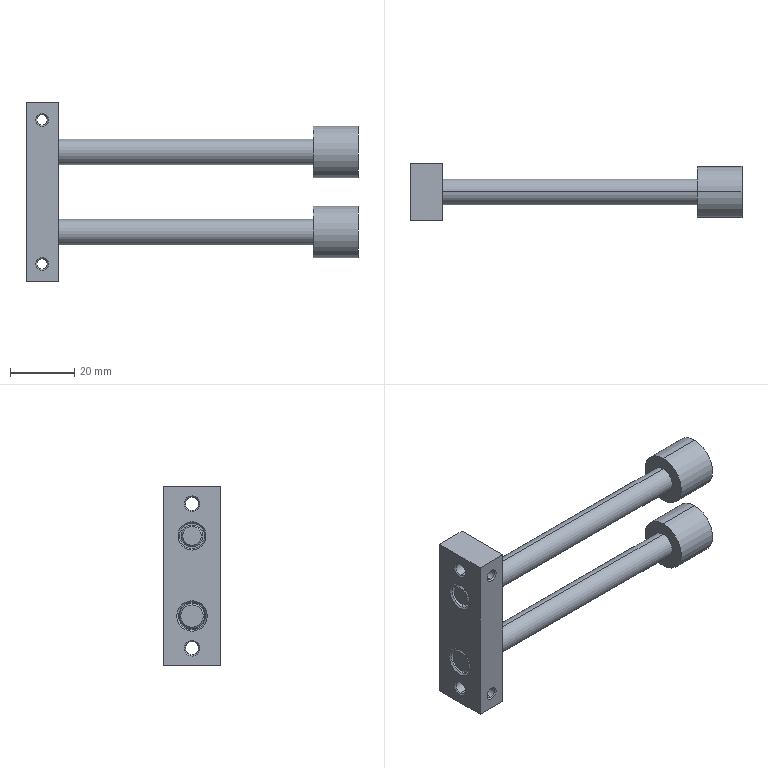Part | SolidWorks | features BaseBody 1 | 1 solid | 71 faces | box 103.6 x 18 x 56 mm | volume 23014 mm3 | cylinder 30 | cone 26 | plane 15 | commonest cylinder face diameters 3.242 x8 8 x6 4.134 x4 16 x4 6 x2 6.8 x2